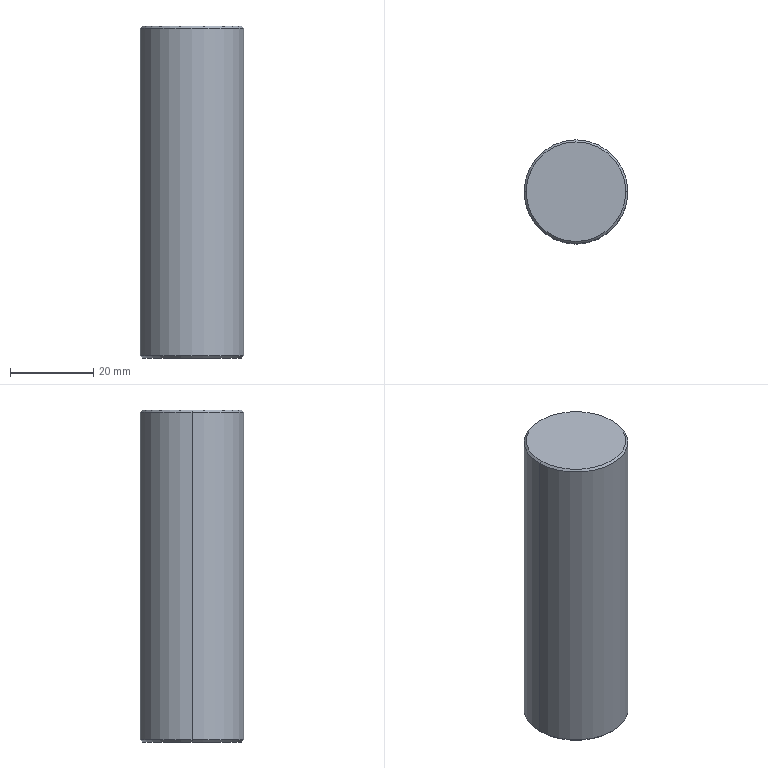Part | SolidWorks | features Revolution 1 | 1 solid | 8 faces | box 25 x 25 x 80 mm | volume 39251 mm3 | cone 4 | cylinder 2 | plane 2 | commonest cylinder face diameters 25 x2
STEP:
#1=CARTESIAN_POINT('',(-12.,0.,0.));
#2=VERTEX_POINT('',#1);
#3=CARTESIAN_POINT('',(12.,0.,0.));
#4=VERTEX_POINT('',#3);
#5=CARTESIAN_POINT('',(0.,0.,0.));
#6=DIRECTION('',(0.,0.,-1.));
#7=DIRECTION('',(-1.,0.,0.));
#8=AXIS2_PLACEMENT_3D('',#5,#6,#7);
#9=CIRCLE('',#8,12.);
#10=EDGE_CURVE('',#2,#4,#9,.T.);
#11=ORIENTED_EDGE('',*,*,#10,.F.);
#12=CARTESIAN_POINT('',(-12.5,0.,0.5));
#13=VERTEX_POINT('',#12);
#14=CARTESIAN_POINT('',(-12.,0.,0.));
#15=DIRECTION('',(-0.7071,0.,0.7071));
#16=VECTOR('',#15,1000.);
#17=LINE('',#14,#16);
#18=EDGE_CURVE('',#2,#13,#17,.T.);
#19=ORIENTED_EDGE('',*,*,#18,.T.);
#20=CARTESIAN_POINT('',(12.5,0.,0.5));
#21=VERTEX_POINT('',#20);
#22=CARTESIAN_POINT('',(0.,0.,0.5));
#23=DIRECTION('',(0.,0.,-1.));
#24=DIRECTION('',(-1.,0.,0.));
#25=AXIS2_PLACEMENT_3D('',#22,#23,#24);
#26=CIRCLE('',#25,12.5);
#27=EDGE_CURVE('',#13,#21,#26,.T.);
#28=ORIENTED_EDGE('',*,*,#27,.T.);
#29=CARTESIAN_POINT('',(12.,0.,0.));
#30=DIRECTION('',(0.7071,0.,0.7071));
#31=VECTOR('',#30,1000.);
#32=LINE('',#29,#31);
#33=EDGE_CURVE('',#4,#21,#32,.T.);
#34=ORIENTED_EDGE('',*,*,#33,.F.);
#35=EDGE_LOOP('',(#11,#19,#28,#34));
#36=FACE_OUTER_BOUND('',#35,.T.);
#37=CARTESIAN_POINT('',(0.,0.,0.));
#38=DIRECTION('',(0.,0.,1.));
#39=DIRECTION('',(1.,0.,0.));
#40=AXIS2_PLACEMENT_3D('',#37,#38,#39);
#41=CONICAL_SURFACE('',#40,12.,0.7854);
#42=ADVANCED_FACE('',(#36),#41,.T.);
#43=CARTESIAN_POINT('',(-12.5,0.,79.5));
#44=VERTEX_POINT('',#43);
#45=CARTESIAN_POINT('',(12.5,0.,79.5));
#46=VERTEX_POINT('',#45);
#47=CARTESIAN_POINT('',(0.,0.,79.5));
#48=DIRECTION('',(0.,0.,-1.));
#49=DIRECTION('',(-1.,0.,0.));
#50=AXIS2_PLACEMENT_3D('',#47,#48,#49);
#51=CIRCLE('',#50,12.5);
#52=EDGE_CURVE('',#44,#46,#51,.T.);
#53=ORIENTED_EDGE('',*,*,#52,.T.);
#54=CARTESIAN_POINT('',(12.5,0.,80.));
#55=DIRECTION('',(0.,0.,-1.));
#56=VECTOR('',#55,1000.);
#57=LINE('',#54,#56);
#58=EDGE_CURVE('',#46,#21,#57,.T.);
#59=ORIENTED_EDGE('',*,*,#58,.T.);
#60=ORIENTED_EDGE('',*,*,#27,.F.);
#61=CARTESIAN_POINT('',(-12.5,0.,80.));
#62=DIRECTION('',(0.,0.,-1.));
#63=VECTOR('',#62,1000.);
#64=LINE('',#61,#63);
#65=EDGE_CURVE('',#44,#13,#64,.T.);
#66=ORIENTED_EDGE('',*,*,#65,.F.);
#67=EDGE_LOOP('',(#53,#59,#60,#66));
#68=FACE_OUTER_BOUND('',#67,.T.);
#69=CARTESIAN_POINT('',(0.,0.,80.));
#70=DIRECTION('',(0.,0.,-1.));
#71=DIRECTION('',(-1.,0.,0.));
#72=AXIS2_PLACEMENT_3D('',#69,#70,#71);
#73=CYLINDRICAL_SURFACE('',#72,12.5);
#74=ADVANCED_FACE('',(#68),#73,.T.);
#75=CARTESIAN_POINT('',(-12.,0.,80.));
#76=VERTEX_POINT('',#75);
#77=CARTESIAN_POINT('',(12.,0.,80.));
#78=VERTEX_POINT('',#77);
#79=CARTESIAN_POINT('',(0.,0.,80.));
#80=DIRECTION('',(0.,0.,-1.));
#81=DIRECTION('',(-1.,0.,0.));
#82=AXIS2_PLACEMENT_3D('',#79,#80,#81);
#83=CIRCLE('',#82,12.);
#84=EDGE_CURVE('',#76,#78,#83,.T.);
#85=ORIENTED_EDGE('',*,*,#84,.T.);
#86=CARTESIAN_POINT('',(12.5,0.,79.5));
#87=DIRECTION('',(0.7071,0.,-0.7071));
#88=VECTOR('',#87,1000.);
#89=LINE('',#86,#88);
#90=EDGE_CURVE('',#78,#46,#89,.T.);
#91=ORIENTED_EDGE('',*,*,#90,.T.);
#92=ORIENTED_EDGE('',*,*,#52,.F.);
#93=CARTESIAN_POINT('',(-12.5,0.,79.5));
#94=DIRECTION('',(-0.7071,0.,-0.7071));
#95=VECTOR('',#94,1000.);
#96=LINE('',#93,#95);
#97=EDGE_CURVE('',#76,#44,#96,.T.);
#98=ORIENTED_EDGE('',*,*,#97,.F.);
#99=EDGE_LOOP('',(#85,#91,#92,#98));
#100=FACE_OUTER_BOUND('',#99,.T.);
#101=CARTESIAN_POINT('',(0.,0.,79.5));
#102=DIRECTION('',(0.,0.,-1.));
#103=DIRECTION('',(-1.,0.,0.));
#104=AXIS2_PLACEMENT_3D('',#101,#102,#103);
#105=CONICAL_SURFACE('',#104,12.5,0.7854);
#106=ADVANCED_FACE('',(#100),#105,.T.);
#107=ORIENTED_EDGE('',*,*,#90,.F.);
#108=CARTESIAN_POINT('',(0.,0.,80.));
#109=DIRECTION('',(0.,0.,-1.));
#110=DIRECTION('',(-1.,0.,0.));
#111=AXIS2_PLACEMENT_3D('',#108,#109,#110);
#112=CIRCLE('',#111,12.);
#113=EDGE_CURVE('',#78,#76,#112,.T.);
#114=ORIENTED_EDGE('',*,*,#113,.T.);
#115=ORIENTED_EDGE('',*,*,#97,.T.);
#116=CARTESIAN_POINT('',(0.,0.,79.5));
#117=DIRECTION('',(0.,0.,-1.));
#118=DIRECTION('',(-1.,0.,0.));
#119=AXIS2_PLACEMENT_3D('',#116,#117,#118);
#120=CIRCLE('',#119,12.5);
#121=EDGE_CURVE('',#46,#44,#120,.T.);
#122=ORIENTED_EDGE('',*,*,#121,.F.);
#123=EDGE_LOOP('',(#107,#114,#115,#122));
#124=FACE_OUTER_BOUND('',#123,.T.);
#125=CARTESIAN_POINT('',(0.,0.,79.5));
#126=DIRECTION('',(0.,0.,-1.));
#127=DIRECTION('',(-1.,0.,0.));
#128=AXIS2_PLACEMENT_3D('',#125,#126,#127);
#129=CONICAL_SURFACE('',#128,12.5,0.7854);
#130=ADVANCED_FACE('',(#124),#129,.T.);
#131=ORIENTED_EDGE('',*,*,#58,.F.);
#132=ORIENTED_EDGE('',*,*,#121,.T.);
#133=ORIENTED_EDGE('',*,*,#65,.T.);
#134=CARTESIAN_POINT('',(0.,0.,0.5));
#135=DIRECTION('',(0.,0.,-1.));
#136=DIRECTION('',(-1.,0.,0.));
#137=AXIS2_PLACEMENT_3D('',#134,#135,#136);
#138=CIRCLE('',#137,12.5);
#139=EDGE_CURVE('',#21,#13,#138,.T.);
#140=ORIENTED_EDGE('',*,*,#139,.F.);
#141=EDGE_LOOP('',(#131,#132,#133,#140));
#142=FACE_OUTER_BOUND('',#141,.T.);
#143=CARTESIAN_POINT('',(0.,0.,80.));
#144=DIRECTION('',(0.,0.,-1.));
#145=DIRECTION('',(-1.,0.,0.));
#146=AXIS2_PLACEMENT_3D('',#143,#144,#145);
#147=CYLINDRICAL_SURFACE('',#146,12.5);
#148=ADVANCED_FACE('',(#142),#147,.T.);
#149=ORIENTED_EDGE('',*,*,#18,.F.);
#150=CARTESIAN_POINT('',(0.,0.,0.));
#151=DIRECTION('',(0.,0.,-1.));
#152=DIRECTION('',(-1.,0.,0.));
#153=AXIS2_PLACEMENT_3D('',#150,#151,#152);
#154=CIRCLE('',#153,12.);
#155=EDGE_CURVE('',#4,#2,#154,.T.);
#156=ORIENTED_EDGE('',*,*,#155,.F.);
#157=ORIENTED_EDGE('',*,*,#33,.T.);
#158=ORIENTED_EDGE('',*,*,#139,.T.);
#159=EDGE_LOOP('',(#149,#156,#157,#158));
#160=FACE_OUTER_BOUND('',#159,.T.);
#161=CARTESIAN_POINT('',(0.,0.,0.));
#162=DIRECTION('',(0.,0.,1.));
#163=DIRECTION('',(1.,0.,0.));
#164=AXIS2_PLACEMENT_3D('',#161,#162,#163);
#165=CONICAL_SURFACE('',#164,12.,0.7854);
#166=ADVANCED_FACE('',(#160),#165,.T.);
#167=ORIENTED_EDGE('',*,*,#155,.T.);
#168=ORIENTED_EDGE('',*,*,#10,.T.);
#169=EDGE_LOOP('',(#167,#168));
#170=FACE_OUTER_BOUND('',#169,.T.);
#171=CARTESIAN_POINT('',(0.,0.,0.));
#172=DIRECTION('',(0.,0.,-1.));
#173=DIRECTION('',(-1.,0.,0.));
#174=AXIS2_PLACEMENT_3D('',#171,#172,#173);
#175=PLANE('',#174);
#176=ADVANCED_FACE('',(#170),#175,.T.);
#177=ORIENTED_EDGE('',*,*,#84,.F.);
#178=ORIENTED_EDGE('',*,*,#113,.F.);
#179=EDGE_LOOP('',(#177,#178));
#180=FACE_OUTER_BOUND('',#179,.T.);
#181=CARTESIAN_POINT('',(12.,0.,80.));
#182=DIRECTION('',(0.,0.,1.));
#183=DIRECTION('',(1.,0.,0.));
#184=AXIS2_PLACEMENT_3D('',#181,#182,#183);
#185=PLANE('',#184);
#186=ADVANCED_FACE('',(#180),#185,.T.);
#187=CLOSED_SHELL('',(#42,#74,#106,#130,#148,#166,#176,#186));
#188=MANIFOLD_SOLID_BREP('',#187);
#189=CARTESIAN_POINT('',(0.,0.,0.));
#190=DIRECTION('',(0.,0.,1.));
#191=DIRECTION('',(1.,0.,0.));
#192=AXIS2_PLACEMENT_3D('',#189,#190,#191);
#193=(LENGTH_UNIT()NAMED_UNIT(*)SI_UNIT(.MILLI.,.METRE.));
#194=UNCERTAINTY_MEASURE_WITH_UNIT(LENGTH_MEASURE(0.00001),#193,'','');
#195=(NAMED_UNIT(*)PLANE_ANGLE_UNIT()SI_UNIT($,.RADIAN.));
#196=(NAMED_UNIT(*)SI_UNIT($,.STERADIAN.)SOLID_ANGLE_UNIT());
#197=(GEOMETRIC_REPRESENTATION_CONTEXT(3)GLOBAL_UNCERTAINTY_ASSIGNED_CONTEXT((#194))GLOBAL_UNIT_ASSIGNED_CONTEXT((#193,#195,#196))REPRESENTATION_CONTEXT('',''));
#198=ADVANCED_BREP_SHAPE_REPRESENTATION('',(#188,#192),#197);